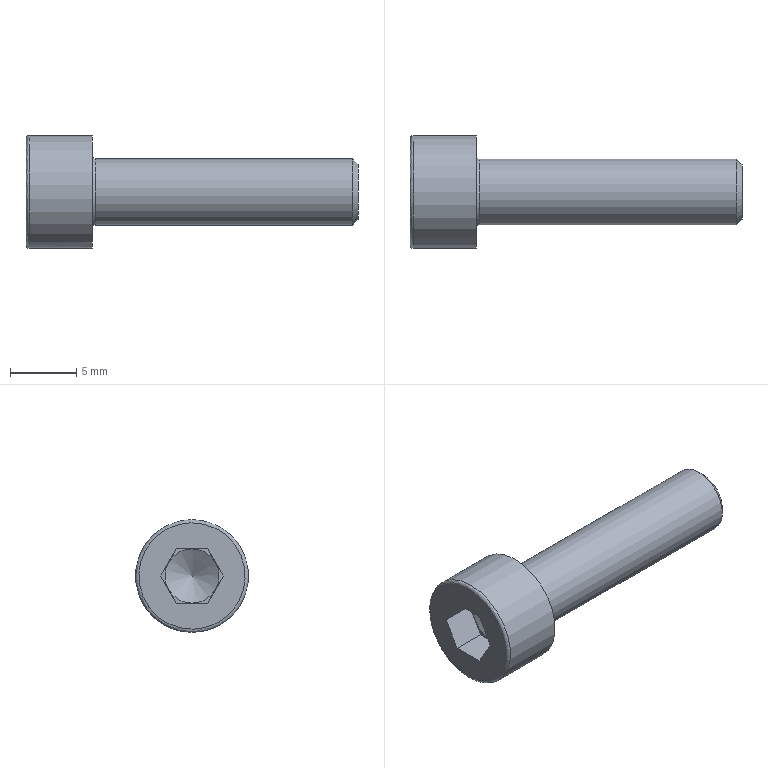Part | STEP file | 1 solid | 21 faces | box 25 x 8.5 x 8.5 mm | volume 633.488 mm3 | plane 15 | cylinder 2 | spline 2 | cone 2 | commonest cylinder face diameters 5 x1 8.5 x1